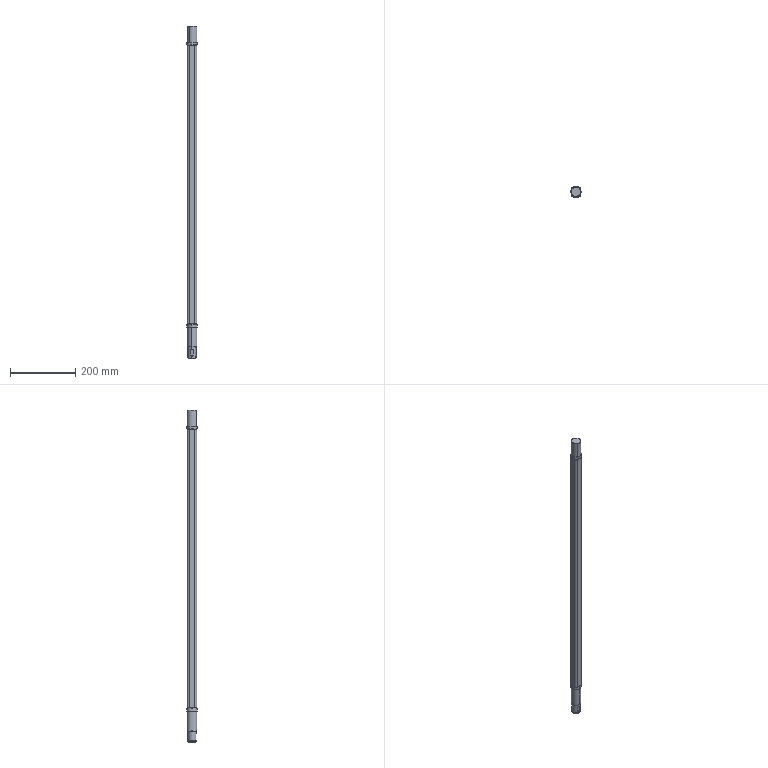Part | SolidWorks | features LayoutProfileFeature 1 | 8 solids | 136 faces | box 32 x 32 x 1016 mm | volume 377179 mm3 | cylinder 52 | plane 48 | cone 32 | spline 4 | commonest cylinder face diameters 15 x20 9 x12 24 x4 25 x4 30 x4 32 x4